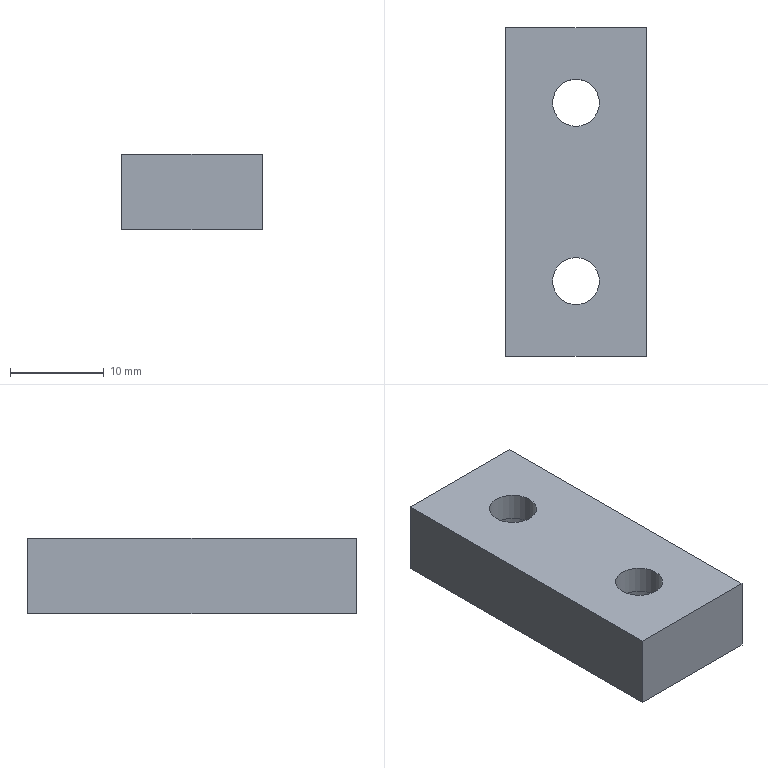Part | NX | features solid 2 | 1 solid | 12 faces | box 15 x 35 x 8 mm | volume 3580 mm3 | plane 8 | cylinder 4 | commonest cylinder face diameters 5 x2 8 x2
STEP:
#1=CARTESIAN_POINT('',(4259.094,-840.622,883.716));
#2=VERTEX_POINT('',#1);
#3=CARTESIAN_POINT('',(4259.094,-840.622,891.716));
#4=VERTEX_POINT('',#3);
#5=CARTESIAN_POINT('',(4259.094,-840.622,891.716));
#6=DIRECTION('',(0.,0.,-1.));
#7=VECTOR('',#6,1000.);
#8=LINE('',#5,#7);
#9=EDGE_CURVE('',#2,#4,#8,.F.);
#10=ORIENTED_EDGE('',*,*,#9,.F.);
#11=CARTESIAN_POINT('',(4244.094,-840.622,883.716));
#12=VERTEX_POINT('',#11);
#13=CARTESIAN_POINT('',(4251.594,-840.622,883.716));
#14=DIRECTION('',(-1.,0.,0.));
#15=VECTOR('',#14,1000.);
#16=LINE('',#13,#15);
#17=EDGE_CURVE('',#2,#12,#16,.T.);
#18=ORIENTED_EDGE('',*,*,#17,.T.);
#19=CARTESIAN_POINT('',(4244.094,-840.622,891.716));
#20=VERTEX_POINT('',#19);
#21=CARTESIAN_POINT('',(4244.094,-840.622,891.716));
#22=DIRECTION('',(0.,0.,1.));
#23=VECTOR('',#22,1000.);
#24=LINE('',#21,#23);
#25=EDGE_CURVE('',#20,#12,#24,.F.);
#26=ORIENTED_EDGE('',*,*,#25,.F.);
#27=CARTESIAN_POINT('',(4251.594,-840.622,891.716));
#28=DIRECTION('',(-1.,0.,0.));
#29=VECTOR('',#28,1000.);
#30=LINE('',#27,#29);
#31=EDGE_CURVE('',#4,#20,#30,.T.);
#32=ORIENTED_EDGE('',*,*,#31,.F.);
#33=EDGE_LOOP('',(#10,#18,#26,#32));
#34=FACE_BOUND('',#33,.T.);
#35=CARTESIAN_POINT('',(4264.094,-840.622,903.716));
#36=DIRECTION('',(0.,1.,0.));
#37=DIRECTION('',(0.,0.,1.));
#38=AXIS2_PLACEMENT_3D('',#35,#36,#37);
#39=PLANE('',#38);
#40=ADVANCED_FACE('',(#34),#39,.T.);
#41=CARTESIAN_POINT('',(4254.094,-848.622,891.716));
#42=VERTEX_POINT('',#41);
#43=CARTESIAN_POINT('',(4251.594,-848.622,891.716));
#44=DIRECTION('',(0.,0.,1.));
#45=DIRECTION('',(1.,0.,0.));
#46=AXIS2_PLACEMENT_3D('',#43,#44,#45);
#47=CIRCLE('',#46,2.5);
#48=EDGE_CURVE('',#42,#42,#47,.T.);
#49=ORIENTED_EDGE('',*,*,#48,.F.);
#50=EDGE_LOOP('',(#49));
#51=FACE_BOUND('',#50,.T.);
#52=CARTESIAN_POINT('',(4254.094,-867.622,891.716));
#53=VERTEX_POINT('',#52);
#54=CARTESIAN_POINT('',(4251.594,-867.622,891.716));
#55=DIRECTION('',(0.,0.,1.));
#56=DIRECTION('',(1.,0.,0.));
#57=AXIS2_PLACEMENT_3D('',#54,#55,#56);
#58=CIRCLE('',#57,2.5);
#59=EDGE_CURVE('',#53,#53,#58,.T.);
#60=ORIENTED_EDGE('',*,*,#59,.F.);
#61=EDGE_LOOP('',(#60));
#62=FACE_BOUND('',#61,.T.);
#63=CARTESIAN_POINT('',(4244.094,-875.622,891.716));
#64=VERTEX_POINT('',#63);
#65=CARTESIAN_POINT('',(4259.094,-875.622,891.716));
#66=VERTEX_POINT('',#65);
#67=CARTESIAN_POINT('',(4264.094,-875.622,891.716));
#68=DIRECTION('',(1.,0.,0.));
#69=VECTOR('',#68,1000.);
#70=LINE('',#67,#69);
#71=EDGE_CURVE('',#64,#66,#70,.T.);
#72=ORIENTED_EDGE('',*,*,#71,.T.);
#73=CARTESIAN_POINT('',(4259.094,-922.622,891.716));
#74=DIRECTION('',(0.,1.,0.));
#75=VECTOR('',#74,1000.);
#76=LINE('',#73,#75);
#77=EDGE_CURVE('',#4,#66,#76,.F.);
#78=ORIENTED_EDGE('',*,*,#77,.F.);
#79=ORIENTED_EDGE('',*,*,#31,.T.);
#80=CARTESIAN_POINT('',(4244.094,-865.622,891.716));
#81=DIRECTION('',(0.,-1.,0.));
#82=VECTOR('',#81,1000.);
#83=LINE('',#80,#82);
#84=EDGE_CURVE('',#64,#20,#83,.F.);
#85=ORIENTED_EDGE('',*,*,#84,.F.);
#86=EDGE_LOOP('',(#72,#78,#79,#85));
#87=FACE_BOUND('',#86,.T.);
#88=CARTESIAN_POINT('',(4251.594,-865.622,891.716));
#89=DIRECTION('',(0.,0.,1.));
#90=DIRECTION('',(1.,0.,0.));
#91=AXIS2_PLACEMENT_3D('',#88,#89,#90);
#92=PLANE('',#91);
#93=ADVANCED_FACE('',(#51,#62,#87),#92,.T.);
#94=CARTESIAN_POINT('',(4255.594,-848.622,883.716));
#95=VERTEX_POINT('',#94);
#96=CARTESIAN_POINT('',(4251.594,-848.622,883.716));
#97=DIRECTION('',(0.,0.,1.));
#98=DIRECTION('',(1.,0.,0.));
#99=AXIS2_PLACEMENT_3D('',#96,#97,#98);
#100=CIRCLE('',#99,4.);
#101=EDGE_CURVE('',#95,#95,#100,.T.);
#102=ORIENTED_EDGE('',*,*,#101,.T.);
#103=EDGE_LOOP('',(#102));
#104=FACE_BOUND('',#103,.T.);
#105=CARTESIAN_POINT('',(4255.594,-867.622,883.716));
#106=VERTEX_POINT('',#105);
#107=CARTESIAN_POINT('',(4251.594,-867.622,883.716));
#108=DIRECTION('',(0.,0.,1.));
#109=DIRECTION('',(1.,0.,0.));
#110=AXIS2_PLACEMENT_3D('',#107,#108,#109);
#111=CIRCLE('',#110,4.);
#112=EDGE_CURVE('',#106,#106,#111,.T.);
#113=ORIENTED_EDGE('',*,*,#112,.T.);
#114=EDGE_LOOP('',(#113));
#115=FACE_BOUND('',#114,.T.);
#116=CARTESIAN_POINT('',(4259.094,-875.622,883.716));
#117=VERTEX_POINT('',#116);
#118=CARTESIAN_POINT('',(4259.094,-922.622,883.716));
#119=DIRECTION('',(0.,1.,0.));
#120=VECTOR('',#119,1000.);
#121=LINE('',#118,#120);
#122=EDGE_CURVE('',#2,#117,#121,.F.);
#123=ORIENTED_EDGE('',*,*,#122,.T.);
#124=CARTESIAN_POINT('',(4244.094,-875.622,883.716));
#125=VERTEX_POINT('',#124);
#126=CARTESIAN_POINT('',(4264.094,-875.622,883.716));
#127=DIRECTION('',(1.,0.,0.));
#128=VECTOR('',#127,1000.);
#129=LINE('',#126,#128);
#130=EDGE_CURVE('',#125,#117,#129,.T.);
#131=ORIENTED_EDGE('',*,*,#130,.F.);
#132=CARTESIAN_POINT('',(4244.094,-865.622,883.716));
#133=DIRECTION('',(0.,-1.,0.));
#134=VECTOR('',#133,1000.);
#135=LINE('',#132,#134);
#136=EDGE_CURVE('',#125,#12,#135,.F.);
#137=ORIENTED_EDGE('',*,*,#136,.T.);
#138=ORIENTED_EDGE('',*,*,#17,.F.);
#139=EDGE_LOOP('',(#123,#131,#137,#138));
#140=FACE_BOUND('',#139,.T.);
#141=CARTESIAN_POINT('',(4251.594,-865.622,883.716));
#142=DIRECTION('',(0.,0.,1.));
#143=DIRECTION('',(1.,0.,0.));
#144=AXIS2_PLACEMENT_3D('',#141,#142,#143);
#145=PLANE('',#144);
#146=ADVANCED_FACE('',(#104,#115,#140),#145,.F.);
#147=CARTESIAN_POINT('',(4259.094,-875.622,903.716));
#148=DIRECTION('',(0.,0.,1.));
#149=VECTOR('',#148,1000.);
#150=LINE('',#147,#149);
#151=EDGE_CURVE('',#66,#117,#150,.F.);
#152=ORIENTED_EDGE('',*,*,#151,.T.);
#153=ORIENTED_EDGE('',*,*,#122,.F.);
#154=ORIENTED_EDGE('',*,*,#9,.T.);
#155=ORIENTED_EDGE('',*,*,#77,.T.);
#156=EDGE_LOOP('',(#152,#153,#154,#155));
#157=FACE_BOUND('',#156,.T.);
#158=CARTESIAN_POINT('',(4259.094,-922.622,891.716));
#159=DIRECTION('',(-1.,0.,0.));
#160=DIRECTION('',(0.,-1.,0.));
#161=AXIS2_PLACEMENT_3D('',#158,#159,#160);
#162=PLANE('',#161);
#163=ADVANCED_FACE('',(#157),#162,.F.);
#164=CARTESIAN_POINT('',(4244.094,-875.622,903.716));
#165=DIRECTION('',(0.,0.,-1.));
#166=VECTOR('',#165,1000.);
#167=LINE('',#164,#166);
#168=EDGE_CURVE('',#125,#64,#167,.F.);
#169=ORIENTED_EDGE('',*,*,#168,.T.);
#170=ORIENTED_EDGE('',*,*,#84,.T.);
#171=ORIENTED_EDGE('',*,*,#25,.T.);
#172=ORIENTED_EDGE('',*,*,#136,.F.);
#173=EDGE_LOOP('',(#169,#170,#171,#172));
#174=FACE_BOUND('',#173,.T.);
#175=CARTESIAN_POINT('',(4244.094,-865.622,891.716));
#176=DIRECTION('',(1.,0.,0.));
#177=DIRECTION('',(0.,1.,0.));
#178=AXIS2_PLACEMENT_3D('',#175,#176,#177);
#179=PLANE('',#178);
#180=ADVANCED_FACE('',(#174),#179,.F.);
#181=ORIENTED_EDGE('',*,*,#151,.F.);
#182=ORIENTED_EDGE('',*,*,#71,.F.);
#183=ORIENTED_EDGE('',*,*,#168,.F.);
#184=ORIENTED_EDGE('',*,*,#130,.T.);
#185=EDGE_LOOP('',(#181,#182,#183,#184));
#186=FACE_BOUND('',#185,.T.);
#187=CARTESIAN_POINT('',(4264.094,-875.622,903.716));
#188=DIRECTION('',(0.,1.,0.));
#189=DIRECTION('',(0.,0.,1.));
#190=AXIS2_PLACEMENT_3D('',#187,#188,#189);
#191=PLANE('',#190);
#192=ADVANCED_FACE('',(#186),#191,.F.);
#193=CARTESIAN_POINT('',(4251.594,-863.622,888.716));
#194=VERTEX_POINT('',#193);
#195=CARTESIAN_POINT('',(4251.594,-867.622,888.716));
#196=DIRECTION('',(0.,0.,-1.));
#197=DIRECTION('',(0.,1.,0.));
#198=AXIS2_PLACEMENT_3D('',#195,#196,#197);
#199=CIRCLE('',#198,4.);
#200=EDGE_CURVE('',#194,#194,#199,.F.);
#201=ORIENTED_EDGE('',*,*,#200,.T.);
#202=EDGE_LOOP('',(#201));
#203=FACE_BOUND('',#202,.T.);
#204=ORIENTED_EDGE('',*,*,#112,.F.);
#205=EDGE_LOOP('',(#204));
#206=FACE_BOUND('',#205,.T.);
#207=CARTESIAN_POINT('',(4251.594,-867.622,888.716));
#208=DIRECTION('',(0.,0.,-1.));
#209=DIRECTION('',(-1.,0.,0.));
#210=AXIS2_PLACEMENT_3D('',#207,#208,#209);
#211=CYLINDRICAL_SURFACE('',#210,4.);
#212=ADVANCED_FACE('',(#203,#206),#211,.F.);
#213=ORIENTED_EDGE('',*,*,#59,.T.);
#214=EDGE_LOOP('',(#213));
#215=FACE_BOUND('',#214,.T.);
#216=CARTESIAN_POINT('',(4249.094,-867.622,888.716));
#217=VERTEX_POINT('',#216);
#218=CARTESIAN_POINT('',(4251.594,-867.622,888.716));
#219=DIRECTION('',(0.,0.,-1.));
#220=DIRECTION('',(-1.,0.,0.));
#221=AXIS2_PLACEMENT_3D('',#218,#219,#220);
#222=CIRCLE('',#221,2.5);
#223=EDGE_CURVE('',#217,#217,#222,.T.);
#224=ORIENTED_EDGE('',*,*,#223,.T.);
#225=EDGE_LOOP('',(#224));
#226=FACE_BOUND('',#225,.T.);
#227=CARTESIAN_POINT('',(4251.594,-867.622,892.716));
#228=DIRECTION('',(0.,0.,-1.));
#229=DIRECTION('',(-1.,0.,0.));
#230=AXIS2_PLACEMENT_3D('',#227,#228,#229);
#231=CYLINDRICAL_SURFACE('',#230,2.5);
#232=ADVANCED_FACE('',(#215,#226),#231,.F.);
#233=ORIENTED_EDGE('',*,*,#223,.F.);
#234=EDGE_LOOP('',(#233));
#235=FACE_BOUND('',#234,.T.);
#236=ORIENTED_EDGE('',*,*,#200,.F.);
#237=EDGE_LOOP('',(#236));
#238=FACE_BOUND('',#237,.T.);
#239=CARTESIAN_POINT('',(4251.594,-867.622,888.716));
#240=DIRECTION('',(0.,0.,-1.));
#241=DIRECTION('',(-1.,0.,0.));
#242=AXIS2_PLACEMENT_3D('',#239,#240,#241);
#243=PLANE('',#242);
#244=ADVANCED_FACE('',(#235,#238),#243,.T.);
#245=CARTESIAN_POINT('',(4251.594,-844.622,888.716));
#246=VERTEX_POINT('',#245);
#247=CARTESIAN_POINT('',(4251.594,-848.622,888.716));
#248=DIRECTION('',(0.,0.,-1.));
#249=DIRECTION('',(0.,1.,0.));
#250=AXIS2_PLACEMENT_3D('',#247,#248,#249);
#251=CIRCLE('',#250,4.);
#252=EDGE_CURVE('',#246,#246,#251,.F.);
#253=ORIENTED_EDGE('',*,*,#252,.T.);
#254=EDGE_LOOP('',(#253));
#255=FACE_BOUND('',#254,.T.);
#256=ORIENTED_EDGE('',*,*,#101,.F.);
#257=EDGE_LOOP('',(#256));
#258=FACE_BOUND('',#257,.T.);
#259=CARTESIAN_POINT('',(4251.594,-848.622,888.716));
#260=DIRECTION('',(0.,0.,-1.));
#261=DIRECTION('',(-1.,0.,0.));
#262=AXIS2_PLACEMENT_3D('',#259,#260,#261);
#263=CYLINDRICAL_SURFACE('',#262,4.);
#264=ADVANCED_FACE('',(#255,#258),#263,.F.);
#265=ORIENTED_EDGE('',*,*,#48,.T.);
#266=EDGE_LOOP('',(#265));
#267=FACE_BOUND('',#266,.T.);
#268=CARTESIAN_POINT('',(4249.094,-848.622,888.716));
#269=VERTEX_POINT('',#268);
#270=CARTESIAN_POINT('',(4251.594,-848.622,888.716));
#271=DIRECTION('',(0.,0.,-1.));
#272=DIRECTION('',(-1.,0.,0.));
#273=AXIS2_PLACEMENT_3D('',#270,#271,#272);
#274=CIRCLE('',#273,2.5);
#275=EDGE_CURVE('',#269,#269,#274,.T.);
#276=ORIENTED_EDGE('',*,*,#275,.T.);
#277=EDGE_LOOP('',(#276));
#278=FACE_BOUND('',#277,.T.);
#279=CARTESIAN_POINT('',(4251.594,-848.622,892.716));
#280=DIRECTION('',(0.,0.,-1.));
#281=DIRECTION('',(-1.,0.,0.));
#282=AXIS2_PLACEMENT_3D('',#279,#280,#281);
#283=CYLINDRICAL_SURFACE('',#282,2.5);
#284=ADVANCED_FACE('',(#267,#278),#283,.F.);
#285=ORIENTED_EDGE('',*,*,#275,.F.);
#286=EDGE_LOOP('',(#285));
#287=FACE_BOUND('',#286,.T.);
#288=ORIENTED_EDGE('',*,*,#252,.F.);
#289=EDGE_LOOP('',(#288));
#290=FACE_BOUND('',#289,.T.);
#291=CARTESIAN_POINT('',(4251.594,-848.622,888.716));
#292=DIRECTION('',(0.,0.,-1.));
#293=DIRECTION('',(-1.,0.,0.));
#294=AXIS2_PLACEMENT_3D('',#291,#292,#293);
#295=PLANE('',#294);
#296=ADVANCED_FACE('',(#287,#290),#295,.T.);
#297=CLOSED_SHELL('',(#40,#93,#146,#163,#180,#192,#212,#232,#244,#264,#284,#296));
#298=MANIFOLD_SOLID_BREP('',#297);
#299=(LENGTH_UNIT()NAMED_UNIT(*)SI_UNIT(.MILLI.,.METRE.));
#300=UNCERTAINTY_MEASURE_WITH_UNIT(LENGTH_MEASURE(0.00001),#299,'','');
#301=(NAMED_UNIT(*)PLANE_ANGLE_UNIT()SI_UNIT($,.RADIAN.));
#302=(NAMED_UNIT(*)SI_UNIT($,.STERADIAN.)SOLID_ANGLE_UNIT());
#303=(GEOMETRIC_REPRESENTATION_CONTEXT(3)GLOBAL_UNCERTAINTY_ASSIGNED_CONTEXT((#300))GLOBAL_UNIT_ASSIGNED_CONTEXT((#299,#301,#302))REPRESENTATION_CONTEXT('',''));
#304=ADVANCED_BREP_SHAPE_REPRESENTATION('',(#298),#303);